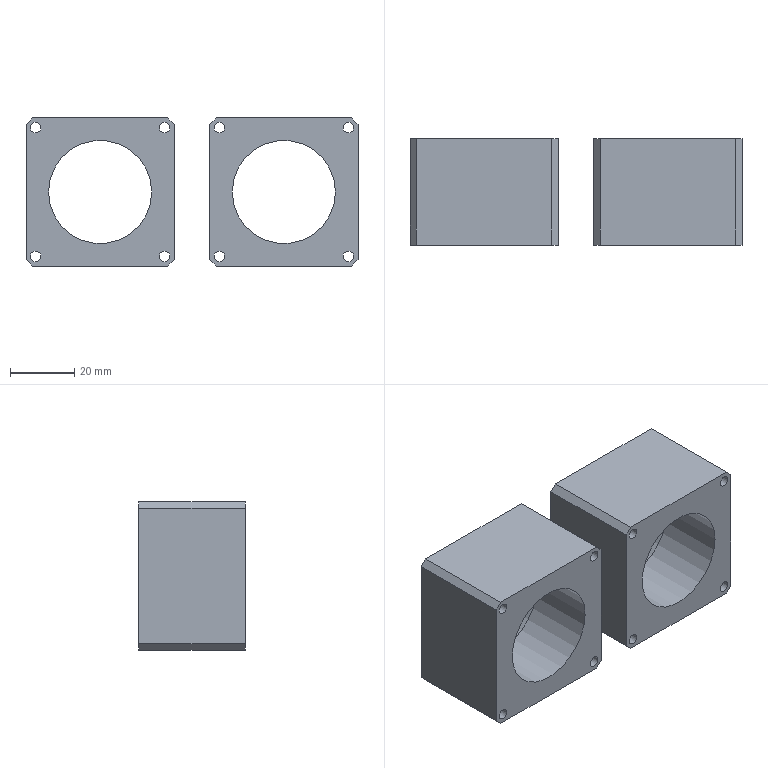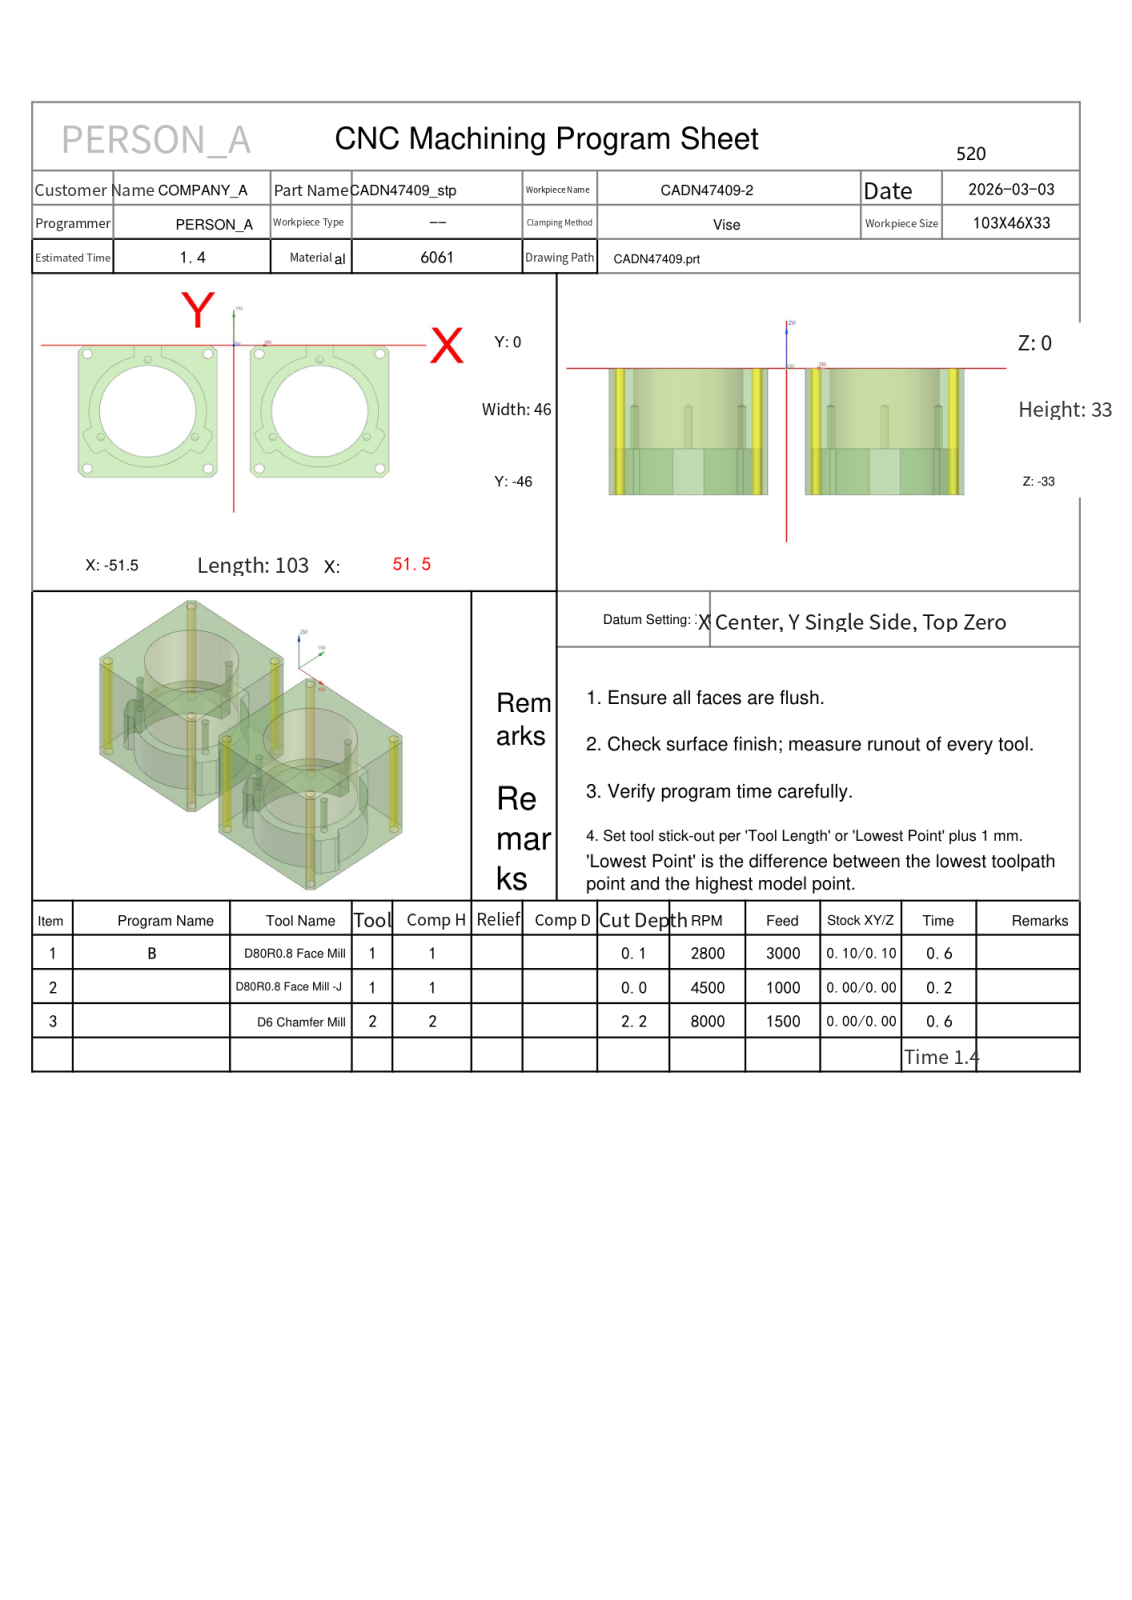NC program | NX | posted by the shop | part box 103 x 33 x 46 mm
Whole program:
%
O0001
(Machine time: 1.91 MIN)
(===Total Tool:2===)
(T1=D80R0.8 Face Mill  D=80.  R=0.8  D-  H01 Z=0.    )
(T2=D6 Chamfer Mill    D=6.   R=0.   D-  H02 Z=-2.2  )
G80 G90 G17 G49 G40
G91 G28 Z0
M01
N1 T01 M06
(D80R0.8 Face Mill   D=80. R=0.8 H=01 ce=0.10 di=0.10)
G00 G90 G54 X-103.597 Y-23.116 M03 S2800
G43 H01 Z50.
M08
Z4.517
G01 Z2.517 F3000.
X-91.597 Y-23.103
X91.597 Y-22.897
X103.597 Y-22.884
Z4.517
G00 X-103.597 Y-23.116
Z4.033
G01 Z2.033
X-91.597 Y-23.103
X91.597 Y-22.897
X103.597 Y-22.884
Z4.033
G00 X-103.597 Y-23.116
Z3.55
G01 Z1.55
X-91.597 Y-23.103
X91.597 Y-22.897
X103.597 Y-22.884
Z3.55
G00 X-103.597 Y-23.116
Z3.067
G01 Z1.067
X-91.597 Y-23.103
X91.597 Y-22.897
X103.597 Y-22.884
Z3.067
G00 Z50.
X-103.597 Y-23.116
Z2.583
G01 Z.583
X-91.597 Y-23.103
X91.597 Y-22.897
X103.597 Y-22.884
Z2.583
G00 Z50.
X-103.597 Y-23.116
Z2.1
G01 Z.1
X-91.597 Y-23.103
X91.597 Y-22.897
X103.597 Y-22.884
Z2.1
G00 Z50.
G91 G28 Z0.0
M05
M09
G91 G28 Z0.0
M01
N2 T01 M06
(D80R0.8 Face Mill -J  D=80. R=0.8 H=01 ce=0.00 di=0.00)
G00 G90 G54 X-103.499 Y-23. M03 S4500
G43 H01 Z50.
M08
Z2.
G01 Z0.0 F1000.
X-91.499
X91.499
X103.499
Z2.
G00 Z50.
G91 G28 Z0.0
M05
M09
G91 G28 Z0.0
M01
N3 T02 M06
(D6 Chamfer Mill   D=6. R=0. H=02 ce=0.00 di=0.00)
G00 G90 G54 X-8.5 Y-43. M03 S8000
G43 H02 Z50.
M08
G98 G81 X-8.5 Y-43. Z-2.2 R3. F1000.
X8.5
X48.5
Y-3.
X8.5
X-8.5
X-48.5
Y-43.
G80
G00 Z50.
G00 G90 X28.114 Y1.227 M03 S6500
Z50.
Z.172
G01 Z-1.2 F1500.
G03 X28.4 Y1.027 I1.286 J1.532
G01 X28.446 Y.997
X28.5 Y1.
X49.5
X49.759 Y.966
X50. Y.866
X50.207 Y.707
X52.207 Y-1.293
X52.366 Y-1.5
X52.466 Y-1.741
X52.5 Y-2.
Y-44.
X52.466 Y-44.259
X52.366 Y-44.5
X52.207 Y-44.707
X50.207 Y-46.707
X50. Y-46.866
X49.759 Y-46.966
X49.5 Y-47.
X7.5
X7.241 Y-46.966
X7. Y-46.866
X6.793 Y-46.707
X4.793 Y-44.707
X4.634 Y-44.5
X4.534 Y-44.259
X4.5 Y-44.
Y-2.
X4.534 Y-1.741
X4.634 Y-1.5
X4.793 Y-1.293
X6.793 Y.707
X7. Y.866
X7.241 Y.966
X7.5 Y1.
X28.5
X28.554 Y.997
X28.6 Y1.027
G03 X28.886 Y1.227 I-1. J1.732
G01 Z.172
G00 Z10.
X48.081 Y-43.494
Z.406
G01 Z-1.2
G03 X48.397 Y-43.641 I1. J1.732
G01 X48.447 Y-43.662
X48.5 Y-43.65
G03 X49.15 Y-43. I0.0 J.65
X48.5 Y-42.35 I-.65 J0.0
X47.85 Y-43. I0.0 J-.65
X48.5 Y-43.65 I.65 J0.0
G01 X48.553 Y-43.662
X48.603 Y-43.641
G03 X48.919 Y-43.494 I-.684 J1.879
G01 Z.402
G00 Z10.
X8.919 Y-42.506
Z.406
G01 Z-1.2
G03 X8.603 Y-42.359 I-1. J-1.732
G01 X8.553 Y-42.338
X8.5 Y-42.35
G03 X7.85 Y-43. I0.0 J-.65
X8.5 Y-43.65 I.65 J0.0
X9.15 Y-43. I0.0 J.65
X8.5 Y-42.35 I-.65 J0.0
G01 X8.447 Y-42.338
X8.397 Y-42.359
G03 X8.081 Y-42.506 I.684 J-1.879
G01 Z.402
G00 Z10.
Y-3.494
Z.402
G01 Z-1.2
G03 X8.397 Y-3.641 I1. J1.732
G01 X8.447 Y-3.662
X8.5 Y-3.65
G03 X9.15 Y-3. I0.0 J.65
X8.5 Y-2.35 I-.65 J0.0
X7.85 Y-3. I0.0 J-.65
X8.5 Y-3.65 I.65 J0.0
G01 X8.553 Y-3.662
X8.603 Y-3.641
G03 X8.919 Y-3.494 I-.684 J1.879
G01 Z.406
G00 Z10.
X28.107 Y-37.787
Z.196
G01 Z-1.2
G03 X28.399 Y-37.977 I1.231 J1.576
G01 X28.446 Y-38.005
X28.5 Y-38.
G03 X43.5 Y-23. I0.0 J15.
X28.5 Y-8. I-15. J0.0
X13.5 Y-23. I0.0 J-15.
X28.5 Y-38. I15. J0.0
G01 X28.554 Y-38.005
X28.601 Y-37.977
G03 X28.893 Y-37.787 I-.939 J1.766
G01 Z.2
G00 Z10.
X48.919 Y-2.506
Z.402
G01 Z-1.2
G03 X48.603 Y-2.359 I-1. J-1.732
G01 X48.553 Y-2.338
X48.5 Y-2.35
G03 X47.85 Y-3. I0.0 J-.65
X48.5 Y-3.65 I.65 J0.0
X49.15 Y-3. I0.0 J.65
X48.5 Y-2.35 I-.65 J0.0
G01 X48.447 Y-2.338
X48.397 Y-2.359
G03 X48.081 Y-2.506 I.684 J-1.879
G01 Z.406
G00 Z10.
X-28.886 Y1.227
Z.172
G01 Z-1.2
G03 X-28.6 Y1.027 I1.286 J1.532
G01 X-28.554 Y.997
X-28.5 Y1.
X-7.5
X-7.241 Y.966
X-7. Y.866
X-6.793 Y.707
X-4.793 Y-1.293
X-4.634 Y-1.5
X-4.534 Y-1.741
X-4.5 Y-2.
Y-44.
X-4.534 Y-44.259
X-4.634 Y-44.5
X-4.793 Y-44.707
X-6.793 Y-46.707
X-7. Y-46.866
X-7.241 Y-46.966
X-7.5 Y-47.
X-49.5
X-49.759 Y-46.966
X-50. Y-46.866
X-50.207 Y-46.707
X-52.207 Y-44.707
X-52.366 Y-44.5
X-52.466 Y-44.259
X-52.5 Y-44.
Y-2.
X-52.466 Y-1.741
X-52.366 Y-1.5
X-52.207 Y-1.293
X-50.207 Y.707
X-50. Y.866
X-49.759 Y.966
X-49.5 Y1.
X-28.5
X-28.446 Y.997
X-28.4 Y1.027
G03 X-28.114 Y1.227 I-1. J1.732
G01 Z.172
G00 Z10.
X-8.919 Y-43.494
Z.406
G01 Z-1.2
G03 X-8.603 Y-43.641 I1. J1.732
G01 X-8.553 Y-43.662
X-8.5 Y-43.65
G03 X-7.85 Y-43. I0.0 J.65
X-8.5 Y-42.35 I-.65 J0.0
X-9.15 Y-43. I0.0 J-.65
X-8.5 Y-43.65 I.65 J0.0
G01 X-8.447 Y-43.662
X-8.397 Y-43.641
G03 X-8.081 Y-43.494 I-.684 J1.879
G01 Z.402
G00 Z10.
X-48.081 Y-42.506
Z.406
G01 Z-1.2
G03 X-48.397 Y-42.359 I-1. J-1.732
G01 X-48.447 Y-42.338
X-48.5 Y-42.35
G03 X-49.15 Y-43. I0.0 J-.65
X-48.5 Y-43.65 I.65 J0.0
X-47.85 Y-43. I0.0 J.65
X-48.5 Y-42.35 I-.65 J0.0
G01 X-48.553 Y-42.338
X-48.603 Y-42.359
G03 X-48.919 Y-42.506 I.684 J-1.879
G01 Z.402
G00 Z10.
X-28.893 Y-37.787
Z.196
G01 Z-1.2
G03 X-28.601 Y-37.977 I1.231 J1.576
G01 X-28.554 Y-38.005
X-28.5 Y-38.
G03 X-13.5 Y-23. I0.0 J15.
X-28.5 Y-8. I-15. J0.0
X-43.5 Y-23. I0.0 J-15.
X-28.5 Y-38. I15. J0.0
G01 X-28.446 Y-38.005
X-28.399 Y-37.977
G03 X-28.107 Y-37.787 I-.939 J1.766
G01 Z.2
G00 Z10.
X-8.081 Y-2.506
Z.402
G01 Z-1.2
G03 X-8.397 Y-2.359 I-1. J-1.732
G01 X-8.447 Y-2.338
X-8.5 Y-2.35
G03 X-9.15 Y-3. I0.0 J-.65
X-8.5 Y-3.65 I.65 J0.0
X-7.85 Y-3. I0.0 J.65
X-8.5 Y-2.35 I-.65 J0.0
G01 X-8.553 Y-2.338
X-8.603 Y-2.359
G03 X-8.919 Y-2.506 I.684 J-1.879
G01 Z.406
G00 Z10.
X-48.919 Y-3.494
Z.402
G01 Z-1.2
G03 X-48.603 Y-3.641 I1. J1.732
G01 X-48.553 Y-3.662
X-48.5 Y-3.65
G03 X-47.85 Y-3. I0.0 J.65
X-48.5 Y-2.35 I-.65 J0.0
X-49.15 Y-3. I0.0 J-.65
X-48.5 Y-3.65 I.65 J0.0
G01 X-48.447 Y-3.662
X-48.397 Y-3.641
G03 X-48.081 Y-3.494 I-.684 J1.879
G01 Z.406
G00 Z50.
M05
M09
G91 G28 Z0.0
G91 G28 Y0.0
M30
%